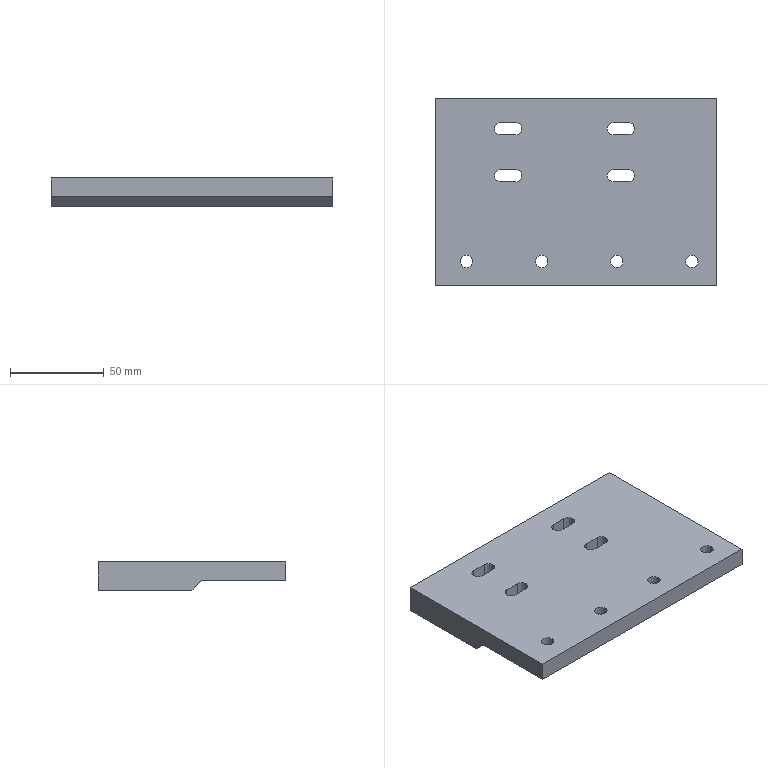Part | STEP file | secondary slingshot input track spacer block 1 | 1 solid | 48 faces | box 150 x 100 x 15 mm | volume 181436 mm3 | cylinder 28 | plane 20 | commonest cylinder face diameters 6.5 x12 6.6 x8 11 x8